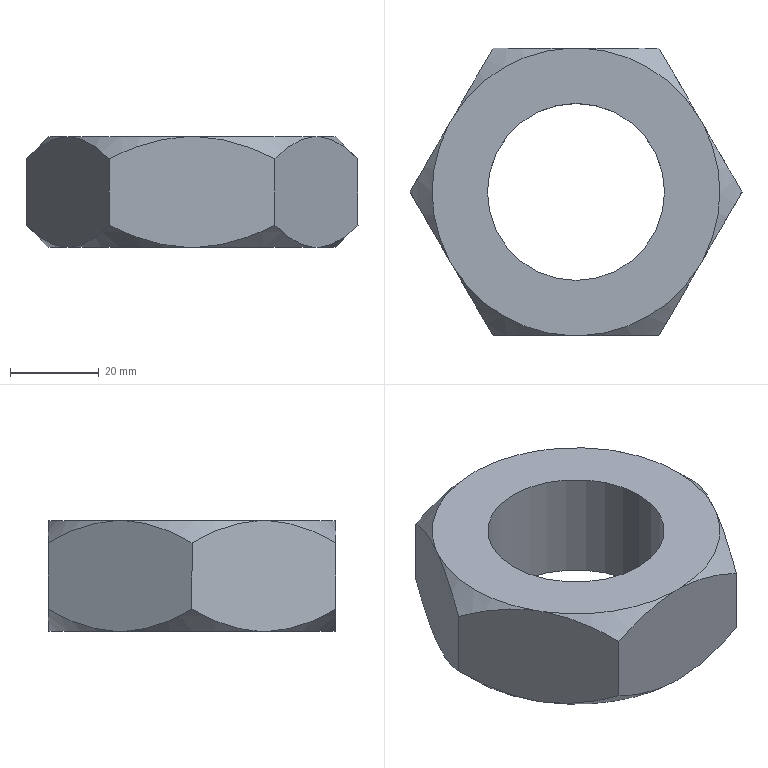Part | Creo | features DATUM PLANE 3, CURVE 2, CHAMFER 1, COORDINATE SYSTEM 1, CUT 1, PROTRUSION 1 | 1 solid | 22 faces | volume 58909 mm3 | cone 12 | plane 8 | cylinder 2 | commonest cylinder face diameters 40 x2